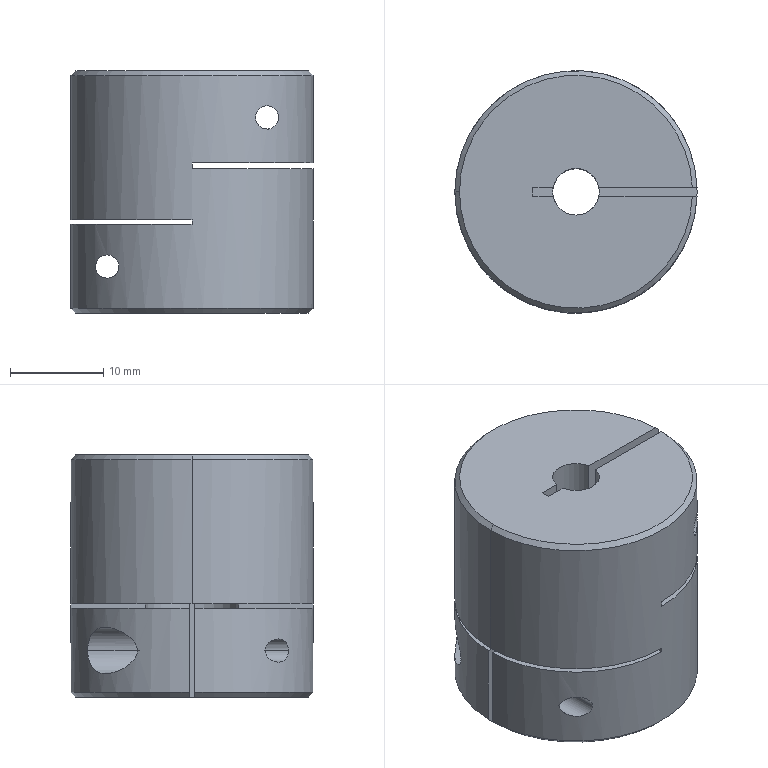Part | SolidWorks | features ICE 6, RevCut 2, Chamfer 1, Extrusion 1 | 1 solid | 49 faces | box 26 x 26 x 26 mm | volume 11774 mm3 | plane 27 | cylinder 18 | cone 4 | commonest cylinder face diameters 2.5 x8 5 x6 10 x2 26 x2